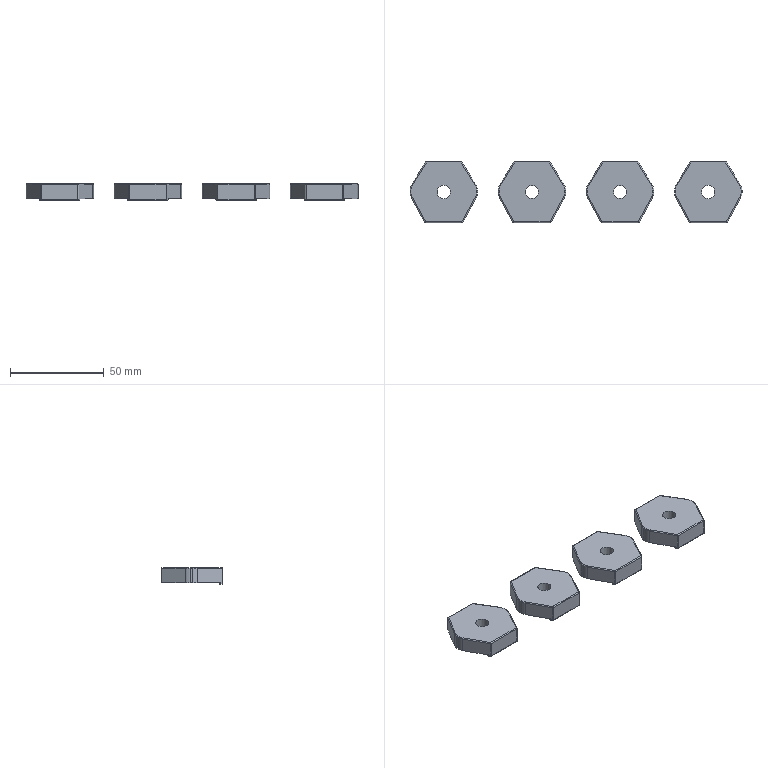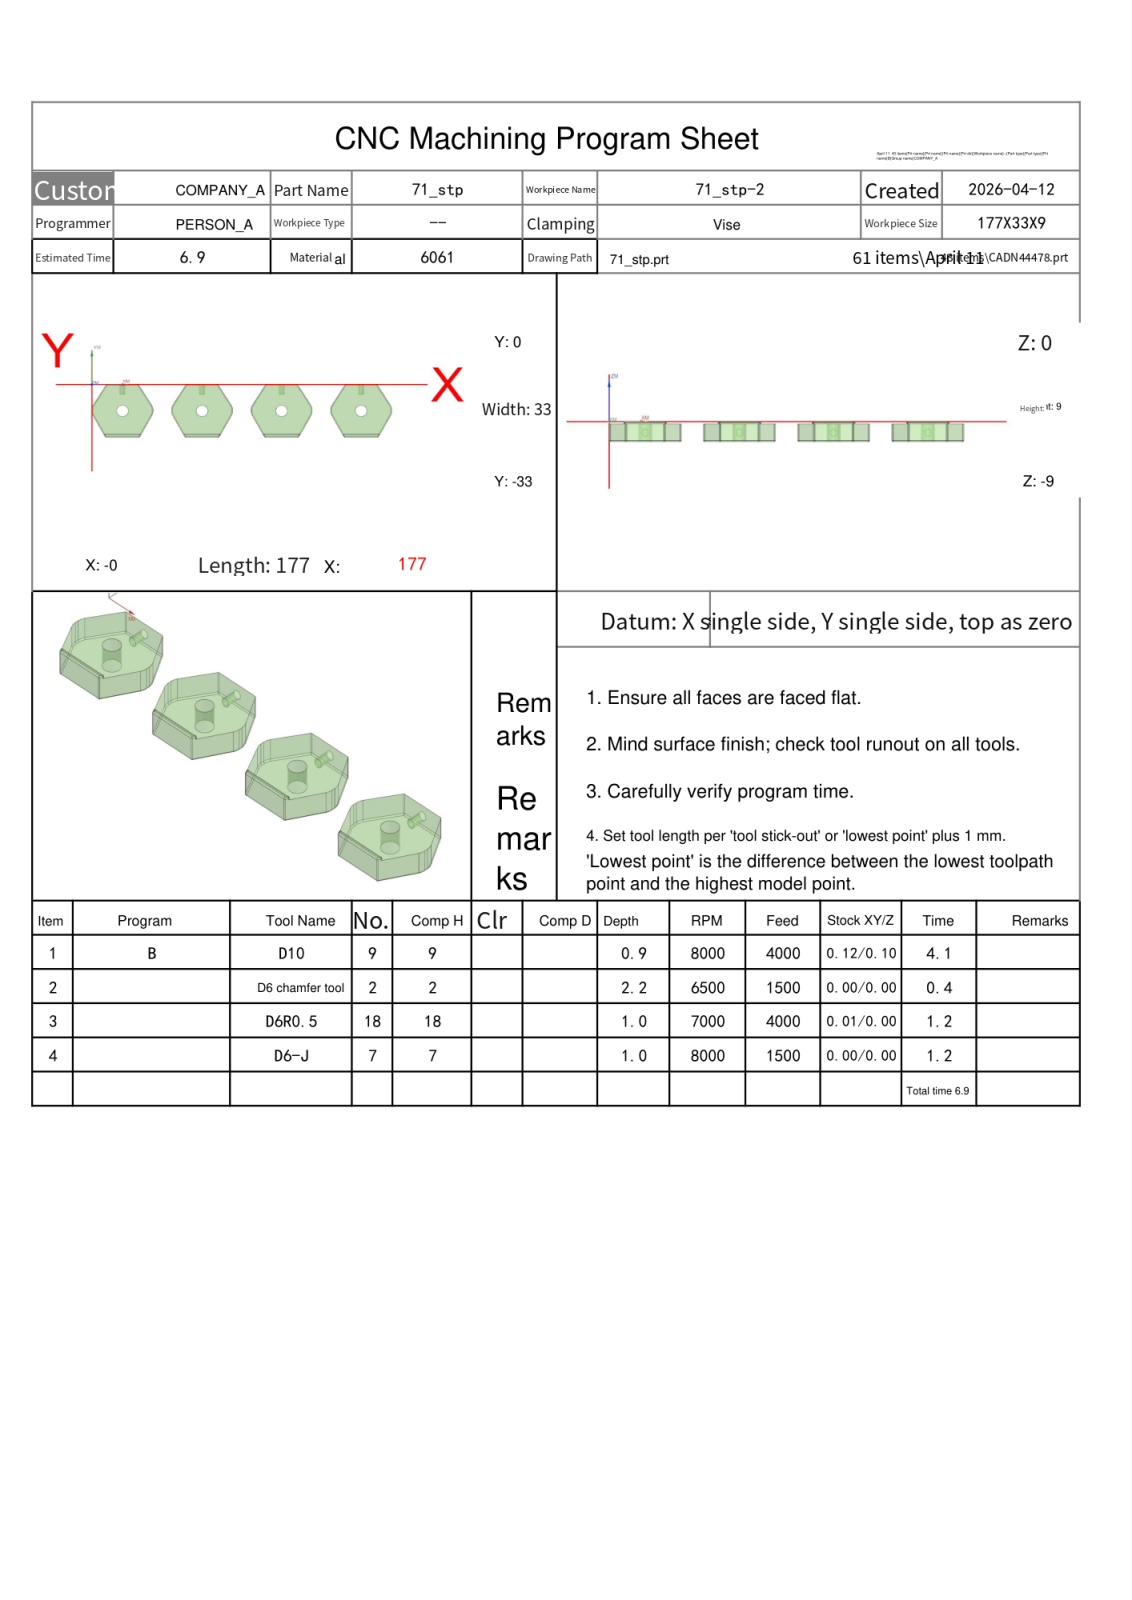NC program | NX | posted by the shop | part box 177 x 33 x 9 mm
Lines 12222 to 12693 of 12693:
N4 T07 M06
(D6-J  D=6. R=0. H=07 ce=0.40 di=0.00)
G00 G90 G54 X2.819 Y-27.3 M03 S7000
G43 H07 Z12.81
M08
Z1.5
G01 Z0.0 F1500.
Y-29.7
G03 X4.019 Y-30.9 I1.2 J0.0
G01 X31.981
G03 X33.181 Y-29.7 I0.0 J1.2
G01 Y-27.3
Z1.5
G00 Z4.
X49.819
Z1.5
G01 Z0.0
Y-29.7
G03 X51.019 Y-30.9 I1.2 J0.0
G01 X78.981
G03 X80.181 Y-29.7 I0.0 J1.2
G01 Y-27.3
Z1.5
G00 Z4.
X96.819
Z1.5
G01 Z0.0
Y-29.7
G03 X98.019 Y-30.9 I1.2 J0.0
G01 X125.981
G03 X127.181 Y-29.7 I0.0 J1.2
G01 Y-27.3
Z1.5
G00 Z4.
X143.819
Z1.5
G01 Z0.0
Y-29.7
G03 X145.019 Y-30.9 I1.2 J0.0
G01 X172.981
G03 X174.181 Y-29.7 I0.0 J1.2
G01 Y-27.3
Z1.5
G00 Z12.81
G00 G90 X29.668 Y3.431 M03 S7000
Z12.81
Z.5
G01 Z-1. F1500.
X29.65 Y.592
G02 X28.45 Y-.601 I-1.2 J.008
G01 X28.442
X28.244 Y-.6
X7.895
G03 X7.383 Y-.887 I0.0 J-.6
G01 X5.982 Y-3.185
X5.938 Y-3.341
G03 X6.238 Y-3.641 I.3 J0.0
G01 X6.254 Y-3.64
G02 X7.756 Y-3.6 I1.502 J-27.86
G01 X28.244
G02 X30.006 Y-3.656 I0.0 J-27.9
X30.48 Y-3.942 I-.038 J-.599
G01 X32.035 Y-6.492
X32.07 Y-6.617
G02 X31.83 Y-6.857 I-.24 J0.0
G01 X31.796 Y-6.855
G03 X28.244 Y-6.6 I-3.552 J-24.645
G01 X7.756
G03 X3.973 Y-6.889 I0.0 J-24.9
X3.552 Y-7.169 I.091 J-.593
G01 X1.757 Y-10.114
X1.73 Y-10.208
G03 X1.91 Y-10.388 I.18 J0.0
G01 X1.958 Y-10.381
G02 X7.756 Y-9.6 I5.798 J-21.119
G01 X28.244
G02 X34.257 Y-10.442 I0.0 J-21.9
X34.604 Y-10.706 I-.165 J-.577
G01 X35.781 Y-12.636
G02 X36.382 Y-14.003 I-4.781 J-2.916
G01 X36.391 Y-14.07
G02 X36.151 Y-14.31 I-.24 J0.0
G01 X36.052 Y-14.288
G03 X28.244 Y-12.6 I-7.808 J-17.212
G01 X7.756
G03 X-.211 Y-14.361 I0.0 J-18.9
X-.553 Y-14.828 I.253 J-.544
X-.6 Y-15.552 I5.553 J-.724
G01 Y-16.968
G03 X-.586 Y-17.36 I5.6 J0.0
X-.227 Y-17.695 I.359 J.025
G01 X-.051 Y-17.648
G02 X7.756 Y-15.6 I7.806 J-13.852
G01 X28.244
G02 X36.139 Y-17.699 I0.0 J-15.9
X36.441 Y-18.219 I-.298 J-.521
G01 X36.422 Y-18.369
G02 X35.924 Y-19.636 I-5.422 J1.401
G01 X35.609 Y-20.218
G02 X35.134 Y-20.5 I-.475 J.257
X34.857 Y-20.424 I0.0 J.54
G03 X28.244 Y-18.6 I-6.613 J-11.076
G01 X7.756
G03 X1.154 Y-20.417 I0.0 J-12.9
X.861 Y-20.933 I.307 J-.515
X.934 Y-21.218 I.6 J0.0
G01 X1.822 Y-22.858
G03 X2.297 Y-23.141 I.475 J.257
X2.579 Y-23.061 I0.0 J.54
G02 X7.756 Y-21.6 I5.177 J-8.439
G01 X28.244
G02 X33.422 Y-23.062 I0.0 J-9.9
X33.708 Y-23.573 I-.314 J-.511
X33.635 Y-23.859 I-.6 J0.0
G01 X32.715 Y-25.558
G02 X32.293 Y-25.81 I-.422 J.229
X32.029 Y-25.731 I0.0 J.48
G03 X28.244 Y-24.6 I-3.785 J-5.769
G01 X7.756
G03 X3.865 Y-25.802 I0.0 J-6.9
X3.604 Y-26.297 I.338 J-.495
G01 X3.614 Y-26.408
X3.994 Y-28.42
G03 X4.583 Y-28.909 I.59 J.111
X5.006 Y-28.734 I0.0 J.6
G02 X7.756 Y-27.6 I2.75 J-2.766
G01 X28.244
G02 X30.994 Y-28.734 I0.0 J-3.9
G03 X31.84 Y-29.083 I.846 J.851
X32.691 Y-28.729 I0.0 J1.2
G01 X34.546 Y-29.735
Z.5
G00 Z3.
X76.668 Y3.431
Z.5
G01 Z-1.
X76.65 Y.592
G02 X75.45 Y-.601 I-1.2 J.008
G01 X75.442
X75.244 Y-.6
X54.895
G03 X54.383 Y-.887 I0.0 J-.6
G01 X52.982 Y-3.185
X52.938 Y-3.341
G03 X53.238 Y-3.641 I.3 J0.0
G01 X53.254 Y-3.64
G02 X54.756 Y-3.6 I1.502 J-27.86
G01 X75.244
G02 X77.006 Y-3.656 I0.0 J-27.9
X77.48 Y-3.942 I-.038 J-.599
G01 X79.035 Y-6.492
X79.07 Y-6.617
G02 X78.83 Y-6.857 I-.24 J0.0
G01 X78.796 Y-6.855
G03 X75.244 Y-6.6 I-3.552 J-24.645
G01 X54.756
G03 X50.973 Y-6.889 I0.0 J-24.9
X50.552 Y-7.169 I.091 J-.593
G01 X48.757 Y-10.114
X48.73 Y-10.208
G03 X48.91 Y-10.388 I.18 J0.0
G01 X48.958 Y-10.381
G02 X54.756 Y-9.6 I5.798 J-21.119
G01 X75.244
G02 X81.257 Y-10.442 I0.0 J-21.9
X81.604 Y-10.706 I-.165 J-.577
G01 X82.781 Y-12.636
G02 X83.382 Y-14.003 I-4.781 J-2.916
G01 X83.391 Y-14.07
G02 X83.151 Y-14.31 I-.24 J0.0
G01 X83.052 Y-14.288
G03 X75.244 Y-12.6 I-7.808 J-17.212
G01 X54.756
G03 X46.789 Y-14.361 I0.0 J-18.9
X46.447 Y-14.827 I.253 J-.544
X46.4 Y-15.552 I5.553 J-.724
G01 Y-16.968
G03 X46.414 Y-17.36 I5.6 J0.0
X46.773 Y-17.695 I.359 J.025
G01 X46.949 Y-17.648
G02 X54.756 Y-15.6 I7.806 J-13.852
G01 X75.244
G02 X83.139 Y-17.699 I0.0 J-15.9
X83.441 Y-18.219 I-.298 J-.521
G01 X83.422 Y-18.369
G02 X82.924 Y-19.636 I-5.422 J1.401
G01 X82.609 Y-20.218
G02 X82.134 Y-20.5 I-.475 J.257
X81.857 Y-20.424 I0.0 J.54
G03 X75.244 Y-18.6 I-6.613 J-11.076
G01 X54.756
G03 X48.154 Y-20.417 I0.0 J-12.9
X47.861 Y-20.933 I.307 J-.515
X47.934 Y-21.218 I.6 J0.0
G01 X48.822 Y-22.858
G03 X49.297 Y-23.141 I.475 J.257
X49.579 Y-23.061 I0.0 J.54
G02 X54.756 Y-21.6 I5.177 J-8.439
G01 X75.244
G02 X80.422 Y-23.062 I0.0 J-9.9
X80.708 Y-23.573 I-.314 J-.511
X80.635 Y-23.859 I-.6 J0.0
G01 X79.715 Y-25.558
G02 X79.293 Y-25.81 I-.422 J.229
X79.029 Y-25.731 I0.0 J.48
G03 X75.244 Y-24.6 I-3.785 J-5.769
G01 X54.756
G03 X50.865 Y-25.802 I0.0 J-6.9
X50.604 Y-26.297 I.339 J-.495
G01 X50.614 Y-26.408
X50.994 Y-28.42
G03 X51.583 Y-28.909 I.59 J.111
X52.006 Y-28.734 I0.0 J.6
G02 X54.756 Y-27.6 I2.75 J-2.766
G01 X75.244
G02 X77.994 Y-28.734 I0.0 J-3.9
G03 X78.84 Y-29.083 I.846 J.851
X79.691 Y-28.729 I0.0 J1.2
G01 X81.546 Y-29.735
Z.5
G00 Z3.
X123.668 Y3.431
Z.5
G01 Z-1.
X123.65 Y.592
G02 X122.45 Y-.601 I-1.2 J.008
G01 X122.442
X122.244 Y-.6
X101.895
G03 X101.383 Y-.887 I0.0 J-.6
G01 X99.982 Y-3.185
X99.938 Y-3.341
G03 X100.238 Y-3.641 I.3 J0.0
G01 X100.254 Y-3.64
G02 X101.756 Y-3.6 I1.502 J-27.86
G01 X122.244
G02 X124.006 Y-3.656 I0.0 J-27.9
X124.48 Y-3.942 I-.038 J-.599
G01 X126.035 Y-6.492
X126.07 Y-6.617
G02 X125.83 Y-6.857 I-.24 J0.0
G01 X125.796 Y-6.855
G03 X122.244 Y-6.6 I-3.552 J-24.645
G01 X101.756
G03 X97.973 Y-6.889 I0.0 J-24.9
X97.552 Y-7.169 I.091 J-.593
G01 X95.757 Y-10.114
X95.73 Y-10.208
G03 X95.91 Y-10.388 I.18 J0.0
G01 X95.958 Y-10.381
G02 X101.756 Y-9.6 I5.798 J-21.119
G01 X122.244
G02 X128.257 Y-10.442 I0.0 J-21.9
X128.604 Y-10.706 I-.165 J-.577
G01 X129.781 Y-12.636
G02 X130.382 Y-14.003 I-4.781 J-2.916
G01 X130.391 Y-14.07
G02 X130.151 Y-14.31 I-.24 J0.0
G01 X130.052 Y-14.288
G03 X122.244 Y-12.6 I-7.808 J-17.212
G01 X101.756
G03 X93.789 Y-14.361 I0.0 J-18.9
X93.447 Y-14.827 I.253 J-.544
X93.4 Y-15.552 I5.553 J-.724
G01 Y-16.968
G03 X93.414 Y-17.36 I5.6 J0.0
X93.773 Y-17.695 I.359 J.025
G01 X93.949 Y-17.648
G02 X101.756 Y-15.6 I7.806 J-13.852
G01 X122.244
G02 X130.139 Y-17.699 I0.0 J-15.9
X130.441 Y-18.219 I-.298 J-.521
G01 X130.422 Y-18.369
G02 X129.924 Y-19.636 I-5.422 J1.401
G01 X129.609 Y-20.218
G02 X129.134 Y-20.5 I-.475 J.257
X128.857 Y-20.424 I0.0 J.54
G03 X122.244 Y-18.6 I-6.613 J-11.076
G01 X101.756
G03 X95.154 Y-20.417 I0.0 J-12.9
X94.861 Y-20.933 I.307 J-.515
X94.934 Y-21.218 I.6 J0.0
G01 X95.822 Y-22.858
G03 X96.297 Y-23.141 I.475 J.257
X96.579 Y-23.061 I0.0 J.54
G02 X101.756 Y-21.6 I5.177 J-8.439
G01 X122.244
G02 X127.422 Y-23.062 I0.0 J-9.9
X127.708 Y-23.573 I-.314 J-.511
X127.635 Y-23.859 I-.6 J0.0
G01 X126.715 Y-25.558
G02 X126.293 Y-25.81 I-.422 J.229
X126.029 Y-25.731 I0.0 J.48
G03 X122.244 Y-24.6 I-3.785 J-5.769
G01 X101.756
G03 X97.865 Y-25.802 I0.0 J-6.9
X97.604 Y-26.297 I.339 J-.495
G01 X97.614 Y-26.408
X97.994 Y-28.42
G03 X98.583 Y-28.909 I.59 J.111
X99.006 Y-28.734 I0.0 J.6
G02 X101.756 Y-27.6 I2.75 J-2.766
G01 X122.244
G02 X124.994 Y-28.734 I0.0 J-3.9
G03 X125.84 Y-29.083 I.846 J.851
X126.691 Y-28.729 I0.0 J1.2
G01 X128.546 Y-29.735
Z.5
G00 Z3.
X170.668 Y3.431
Z.5
G01 Z-1.
X170.65 Y.592
G02 X169.45 Y-.601 I-1.2 J.008
G01 X169.442
X169.244 Y-.6
X148.895
G03 X148.383 Y-.887 I0.0 J-.6
G01 X146.982 Y-3.185
X146.938 Y-3.341
G03 X147.238 Y-3.641 I.3 J0.0
G01 X147.254 Y-3.64
G02 X148.756 Y-3.6 I1.502 J-27.86
G01 X169.244
G02 X171.006 Y-3.656 I0.0 J-27.9
X171.48 Y-3.942 I-.038 J-.599
G01 X173.035 Y-6.492
X173.07 Y-6.617
G02 X172.83 Y-6.857 I-.24 J0.0
G01 X172.796 Y-6.855
G03 X169.244 Y-6.6 I-3.552 J-24.645
G01 X148.756
G03 X144.973 Y-6.889 I0.0 J-24.9
X144.552 Y-7.169 I.091 J-.593
G01 X142.757 Y-10.114
X142.73 Y-10.208
G03 X142.91 Y-10.388 I.18 J0.0
G01 X142.958 Y-10.381
G02 X148.756 Y-9.6 I5.798 J-21.119
G01 X169.244
G02 X175.257 Y-10.442 I0.0 J-21.9
X175.604 Y-10.706 I-.165 J-.577
G01 X176.781 Y-12.636
G02 X177.382 Y-14.003 I-4.781 J-2.916
G01 X177.391 Y-14.07
G02 X177.151 Y-14.31 I-.24 J0.0
G01 X177.052 Y-14.288
G03 X169.244 Y-12.6 I-7.808 J-17.212
G01 X148.756
G03 X140.789 Y-14.361 I0.0 J-18.9
X140.447 Y-14.827 I.253 J-.544
X140.4 Y-15.552 I5.553 J-.724
G01 Y-16.968
G03 X140.414 Y-17.36 I5.6 J0.0
X140.773 Y-17.695 I.359 J.025
G01 X140.949 Y-17.648
G02 X148.756 Y-15.6 I7.806 J-13.852
G01 X169.244
G02 X177.139 Y-17.699 I0.0 J-15.9
X177.441 Y-18.219 I-.298 J-.521
G01 X177.422 Y-18.369
G02 X176.924 Y-19.636 I-5.422 J1.401
G01 X176.609 Y-20.218
G02 X176.134 Y-20.5 I-.475 J.257
X175.857 Y-20.424 I0.0 J.54
G03 X169.244 Y-18.6 I-6.613 J-11.076
G01 X148.756
G03 X142.154 Y-20.417 I0.0 J-12.9
X141.861 Y-20.933 I.307 J-.515
X141.934 Y-21.218 I.6 J0.0
G01 X142.822 Y-22.858
G03 X143.297 Y-23.141 I.475 J.257
X143.579 Y-23.061 I0.0 J.54
G02 X148.756 Y-21.6 I5.177 J-8.439
G01 X169.244
G02 X174.422 Y-23.062 I0.0 J-9.9
X174.708 Y-23.573 I-.314 J-.511
X174.635 Y-23.859 I-.6 J0.0
G01 X173.715 Y-25.558
G02 X173.293 Y-25.81 I-.422 J.229
X173.029 Y-25.731 I0.0 J.48
G03 X169.244 Y-24.6 I-3.785 J-5.769
G01 X148.756
G03 X144.865 Y-25.802 I0.0 J-6.9
X144.604 Y-26.297 I.339 J-.495
G01 X144.614 Y-26.408
X144.994 Y-28.42
G03 X145.583 Y-28.909 I.59 J.111
X146.006 Y-28.734 I0.0 J.6
G02 X148.756 Y-27.6 I2.75 J-2.766
G01 X169.244
G02 X171.994 Y-28.734 I0.0 J-3.9
G03 X172.84 Y-29.083 I.846 J.851
X173.691 Y-28.729 I0.0 J1.2
G01 X175.546 Y-29.735
Z.5
G00 Z12.81
G00 G90 X3.926 Y-34.718 M03 S8000
Z12.81
Z0.0
G01 Z-1. F1000.
G41 D07
X4.103 Y-34.623
G03 X4.734 Y-33.566 I-.568 J1.057
X4.612 Y-33.039 I-1.2 J0.0
G02 X4.256 Y-31.5 I3.144 J1.539
X7.756 Y-28. I3.5 J0.0
G01 X28.244
G02 X31.744 Y-31.5 I0.0 J-3.5
X31.388 Y-33.039 I-3.5 J0.0
G03 X31.266 Y-33.566 I1.078 J-.528
X31.897 Y-34.623 I1.2 J0.0
G01 G40 X32.074 Y-34.718
Z0.0
G00 Z3.
X50.926
Z0.0
G01 Z-1.
G41 D07
X51.103 Y-34.623
G03 X51.734 Y-33.566 I-.568 J1.057
X51.612 Y-33.039 I-1.2 J0.0
G02 X51.256 Y-31.5 I3.144 J1.539
X54.756 Y-28. I3.5 J0.0
G01 X75.244
G02 X78.744 Y-31.5 I0.0 J-3.5
X78.388 Y-33.039 I-3.5 J0.0
G03 X78.266 Y-33.566 I1.078 J-.528
X78.897 Y-34.623 I1.2 J0.0
G01 G40 X79.074 Y-34.718
Z0.0
G00 Z3.
X97.926
Z0.0
G01 Z-1.
G41 D07
X98.103 Y-34.623
G03 X98.734 Y-33.566 I-.568 J1.057
X98.612 Y-33.039 I-1.2 J0.0
G02 X98.256 Y-31.5 I3.144 J1.539
X101.756 Y-28. I3.5 J0.0
G01 X122.244
G02 X125.744 Y-31.5 I0.0 J-3.5
X125.388 Y-33.039 I-3.5 J0.0
G03 X125.266 Y-33.566 I1.078 J-.528
X125.897 Y-34.623 I1.2 J0.0
G01 G40 X126.074 Y-34.718
Z0.0
G00 Z3.
X144.926
Z0.0
G01 Z-1.
G41 D07
X145.103 Y-34.623
G03 X145.734 Y-33.566 I-.568 J1.057
X145.612 Y-33.039 I-1.2 J0.0
G02 X145.256 Y-31.5 I3.144 J1.539
X148.756 Y-28. I3.5 J0.0
G01 X169.244
G02 X172.744 Y-31.5 I0.0 J-3.5
X172.388 Y-33.039 I-3.5 J0.0
G03 X172.266 Y-33.566 I1.078 J-.528
X172.897 Y-34.623 I1.2 J0.0
G01 G40 X173.074 Y-34.718
Z0.0
G00 Z12.81
M05
M09
G91 G28 Z0.0
G91 G28 Y0.0
M30
%